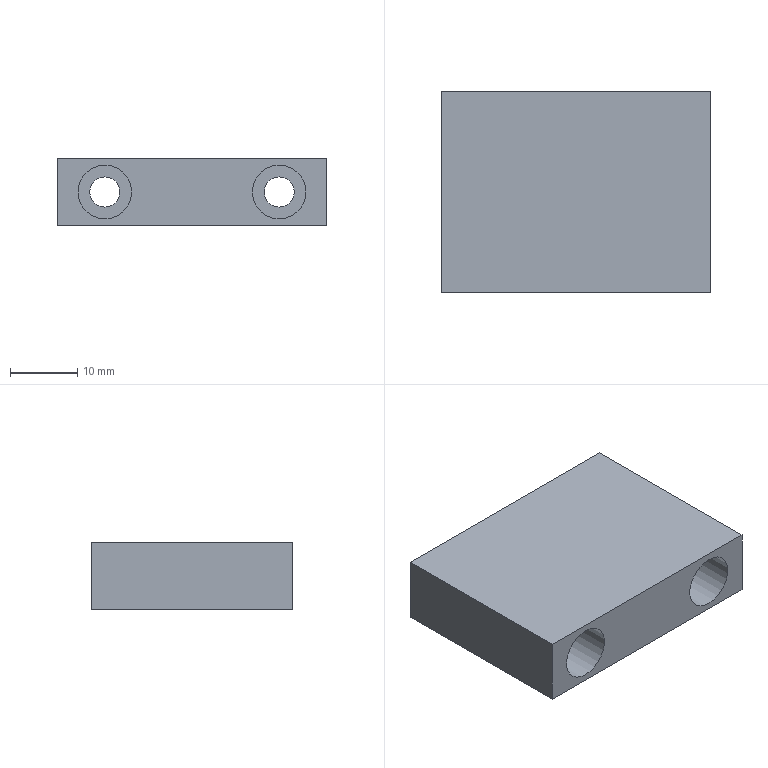Part | STEP file | 1 solid | 12 faces | box 40 x 30 x 10 mm | volume 9671 mm3 | plane 8 | cylinder 4 | commonest cylinder face diameters 4.5 x2 8 x2
STEP:
#1=CARTESIAN_POINT('',(0.,0.,0.));
#2=DIRECTION('',(0.,0.,1.));
#3=DIRECTION('',(1.,0.,0.));
#4=AXIS2_PLACEMENT_3D('',#1,#2,#3);
#5=CARTESIAN_POINT('',(-20.,15.,5.));
#6=VERTEX_POINT('',#5);
#7=CARTESIAN_POINT('',(20.,15.,5.));
#8=VERTEX_POINT('',#7);
#9=CARTESIAN_POINT('',(0.,15.,5.));
#10=DIRECTION('',(1.,0.,0.));
#11=VECTOR('',#10,1.);
#12=LINE('',#9,#11);
#13=CARTESIAN_POINT('',(0.,0.,5.));
#14=DIRECTION('',(0.,0.,-1.));
#15=DIRECTION('',(-1.,0.,0.));
#16=AXIS2_PLACEMENT_3D('',#13,#14,#15);
#17=PLANE('',#16);
#18=CARTESIAN_POINT('',(0.,15.));
#19=DIRECTION('',(-1.,0.));
#20=VECTOR('',#19,1.);
#21=LINE('',#18,#20);
#22=(GEOMETRIC_REPRESENTATION_CONTEXT(2)PARAMETRIC_REPRESENTATION_CONTEXT()REPRESENTATION_CONTEXT('',''));
#23=DEFINITIONAL_REPRESENTATION('',(#21),#22);
#24=PCURVE('',#17,#23);
#25=CARTESIAN_POINT('',(-20.,15.,5.));
#26=DIRECTION('',(0.,-1.,0.));
#27=DIRECTION('',(0.,0.,-1.));
#28=AXIS2_PLACEMENT_3D('',#25,#26,#27);
#29=PLANE('',#28);
#30=CARTESIAN_POINT('',(0.,20.));
#31=DIRECTION('',(0.,1.));
#32=VECTOR('',#31,1.);
#33=LINE('',#30,#32);
#34=(GEOMETRIC_REPRESENTATION_CONTEXT(2)PARAMETRIC_REPRESENTATION_CONTEXT()REPRESENTATION_CONTEXT('',''));
#35=DEFINITIONAL_REPRESENTATION('',(#33),#34);
#36=PCURVE('',#29,#35);
#37=SURFACE_CURVE('',#12,(#24,#36),.PCURVE_S1.);
#38=EDGE_CURVE('',#6,#8,#37,.T.);
#39=ORIENTED_EDGE('',*,*,#38,.F.);
#40=CARTESIAN_POINT('',(-20.,-15.,5.));
#41=VERTEX_POINT('',#40);
#42=CARTESIAN_POINT('',(-20.,0.,5.));
#43=DIRECTION('',(0.,1.,0.));
#44=VECTOR('',#43,1.);
#45=LINE('',#42,#44);
#46=CARTESIAN_POINT('',(20.,0.));
#47=DIRECTION('',(0.,1.));
#48=VECTOR('',#47,1.);
#49=LINE('',#46,#48);
#50=(GEOMETRIC_REPRESENTATION_CONTEXT(2)PARAMETRIC_REPRESENTATION_CONTEXT()REPRESENTATION_CONTEXT('',''));
#51=DEFINITIONAL_REPRESENTATION('',(#49),#50);
#52=PCURVE('',#17,#51);
#53=CARTESIAN_POINT('',(-20.,-15.,5.));
#54=DIRECTION('',(1.,0.,0.));
#55=DIRECTION('',(0.,0.,-1.));
#56=AXIS2_PLACEMENT_3D('',#53,#54,#55);
#57=PLANE('',#56);
#58=CARTESIAN_POINT('',(0.,15.));
#59=DIRECTION('',(0.,1.));
#60=VECTOR('',#59,1.);
#61=LINE('',#58,#60);
#62=(GEOMETRIC_REPRESENTATION_CONTEXT(2)PARAMETRIC_REPRESENTATION_CONTEXT()REPRESENTATION_CONTEXT('',''));
#63=DEFINITIONAL_REPRESENTATION('',(#61),#62);
#64=PCURVE('',#57,#63);
#65=SURFACE_CURVE('',#45,(#52,#64),.PCURVE_S1.);
#66=EDGE_CURVE('',#41,#6,#65,.T.);
#67=ORIENTED_EDGE('',*,*,#66,.F.);
#68=CARTESIAN_POINT('',(20.,-15.,5.));
#69=VERTEX_POINT('',#68);
#70=CARTESIAN_POINT('',(0.,-15.,5.));
#71=DIRECTION('',(-1.,0.,0.));
#72=VECTOR('',#71,1.);
#73=LINE('',#70,#72);
#74=CARTESIAN_POINT('',(0.,-15.));
#75=DIRECTION('',(1.,0.));
#76=VECTOR('',#75,1.);
#77=LINE('',#74,#76);
#78=(GEOMETRIC_REPRESENTATION_CONTEXT(2)PARAMETRIC_REPRESENTATION_CONTEXT()REPRESENTATION_CONTEXT('',''));
#79=DEFINITIONAL_REPRESENTATION('',(#77),#78);
#80=PCURVE('',#17,#79);
#81=CARTESIAN_POINT('',(-20.,-15.,5.));
#82=DIRECTION('',(0.,1.,0.));
#83=DIRECTION('',(0.,0.,1.));
#84=AXIS2_PLACEMENT_3D('',#81,#82,#83);
#85=PLANE('',#84);
#86=CARTESIAN_POINT('',(0.,20.));
#87=DIRECTION('',(0.,-1.));
#88=VECTOR('',#87,1.);
#89=LINE('',#86,#88);
#90=(GEOMETRIC_REPRESENTATION_CONTEXT(2)PARAMETRIC_REPRESENTATION_CONTEXT()REPRESENTATION_CONTEXT('',''));
#91=DEFINITIONAL_REPRESENTATION('',(#89),#90);
#92=PCURVE('',#85,#91);
#93=SURFACE_CURVE('',#73,(#80,#92),.PCURVE_S1.);
#94=EDGE_CURVE('',#69,#41,#93,.T.);
#95=ORIENTED_EDGE('',*,*,#94,.F.);
#96=CARTESIAN_POINT('',(20.,0.,5.));
#97=DIRECTION('',(0.,-1.,0.));
#98=VECTOR('',#97,1.);
#99=LINE('',#96,#98);
#100=CARTESIAN_POINT('',(-20.,0.));
#101=DIRECTION('',(0.,-1.));
#102=VECTOR('',#101,1.);
#103=LINE('',#100,#102);
#104=(GEOMETRIC_REPRESENTATION_CONTEXT(2)PARAMETRIC_REPRESENTATION_CONTEXT()REPRESENTATION_CONTEXT('',''));
#105=DEFINITIONAL_REPRESENTATION('',(#103),#104);
#106=PCURVE('',#17,#105);
#107=CARTESIAN_POINT('',(20.,-15.,5.));
#108=DIRECTION('',(-1.,0.,0.));
#109=DIRECTION('',(0.,0.,1.));
#110=AXIS2_PLACEMENT_3D('',#107,#108,#109);
#111=PLANE('',#110);
#112=CARTESIAN_POINT('',(0.,15.));
#113=DIRECTION('',(0.,-1.));
#114=VECTOR('',#113,1.);
#115=LINE('',#112,#114);
#116=(GEOMETRIC_REPRESENTATION_CONTEXT(2)PARAMETRIC_REPRESENTATION_CONTEXT()REPRESENTATION_CONTEXT('',''));
#117=DEFINITIONAL_REPRESENTATION('',(#115),#116);
#118=PCURVE('',#111,#117);
#119=SURFACE_CURVE('',#99,(#106,#118),.PCURVE_S1.);
#120=EDGE_CURVE('',#8,#69,#119,.T.);
#121=ORIENTED_EDGE('',*,*,#120,.F.);
#122=EDGE_LOOP('',(#39,#67,#95,#121));
#123=FACE_BOUND('',#122,.T.);
#124=ADVANCED_FACE('',(#123),#17,.F.);
#125=CARTESIAN_POINT('',(20.,15.,-5.));
#126=VERTEX_POINT('',#125);
#127=CARTESIAN_POINT('',(20.,15.,5.));
#128=DIRECTION('',(0.,0.,-1.));
#129=VECTOR('',#128,1.);
#130=LINE('',#127,#129);
#131=CARTESIAN_POINT('',(0.,30.));
#132=DIRECTION('',(-1.,0.));
#133=VECTOR('',#132,1.);
#134=LINE('',#131,#133);
#135=(GEOMETRIC_REPRESENTATION_CONTEXT(2)PARAMETRIC_REPRESENTATION_CONTEXT()REPRESENTATION_CONTEXT('',''));
#136=DEFINITIONAL_REPRESENTATION('',(#134),#135);
#137=PCURVE('',#111,#136);
#138=CARTESIAN_POINT('',(0.,40.));
#139=DIRECTION('',(1.,0.));
#140=VECTOR('',#139,1.);
#141=LINE('',#138,#140);
#142=(GEOMETRIC_REPRESENTATION_CONTEXT(2)PARAMETRIC_REPRESENTATION_CONTEXT()REPRESENTATION_CONTEXT('',''));
#143=DEFINITIONAL_REPRESENTATION('',(#141),#142);
#144=PCURVE('',#29,#143);
#145=SURFACE_CURVE('',#130,(#137,#144),.PCURVE_S1.);
#146=EDGE_CURVE('',#8,#126,#145,.T.);
#147=ORIENTED_EDGE('',*,*,#146,.F.);
#148=ORIENTED_EDGE('',*,*,#120,.T.);
#149=CARTESIAN_POINT('',(20.,-15.,-5.));
#150=VERTEX_POINT('',#149);
#151=CARTESIAN_POINT('',(20.,-15.,5.));
#152=DIRECTION('',(0.,0.,1.));
#153=VECTOR('',#152,1.);
#154=LINE('',#151,#153);
#155=CARTESIAN_POINT('',(0.,0.));
#156=DIRECTION('',(1.,0.));
#157=VECTOR('',#156,1.);
#158=LINE('',#155,#157);
#159=(GEOMETRIC_REPRESENTATION_CONTEXT(2)PARAMETRIC_REPRESENTATION_CONTEXT()REPRESENTATION_CONTEXT('',''));
#160=DEFINITIONAL_REPRESENTATION('',(#158),#159);
#161=PCURVE('',#111,#160);
#162=CARTESIAN_POINT('',(0.,40.));
#163=DIRECTION('',(1.,0.));
#164=VECTOR('',#163,1.);
#165=LINE('',#162,#164);
#166=(GEOMETRIC_REPRESENTATION_CONTEXT(2)PARAMETRIC_REPRESENTATION_CONTEXT()REPRESENTATION_CONTEXT('',''));
#167=DEFINITIONAL_REPRESENTATION('',(#165),#166);
#168=PCURVE('',#85,#167);
#169=SURFACE_CURVE('',#154,(#161,#168),.PCURVE_S1.);
#170=EDGE_CURVE('',#150,#69,#169,.T.);
#171=ORIENTED_EDGE('',*,*,#170,.F.);
#172=CARTESIAN_POINT('',(20.,-15.,-5.));
#173=DIRECTION('',(0.,-1.,0.));
#174=VECTOR('',#173,1.);
#175=LINE('',#172,#174);
#176=CARTESIAN_POINT('',(-10.,0.));
#177=DIRECTION('',(0.,-1.));
#178=VECTOR('',#177,1.);
#179=LINE('',#176,#178);
#180=(GEOMETRIC_REPRESENTATION_CONTEXT(2)PARAMETRIC_REPRESENTATION_CONTEXT()REPRESENTATION_CONTEXT('',''));
#181=DEFINITIONAL_REPRESENTATION('',(#179),#180);
#182=PCURVE('',#111,#181);
#183=CARTESIAN_POINT('',(0.,0.,-5.));
#184=DIRECTION('',(0.,0.,-1.));
#185=DIRECTION('',(-1.,0.,0.));
#186=AXIS2_PLACEMENT_3D('',#183,#184,#185);
#187=PLANE('',#186);
#188=CARTESIAN_POINT('',(-20.,-15.));
#189=DIRECTION('',(0.,-1.));
#190=VECTOR('',#189,1.);
#191=LINE('',#188,#190);
#192=(GEOMETRIC_REPRESENTATION_CONTEXT(2)PARAMETRIC_REPRESENTATION_CONTEXT()REPRESENTATION_CONTEXT('',''));
#193=DEFINITIONAL_REPRESENTATION('',(#191),#192);
#194=PCURVE('',#187,#193);
#195=SURFACE_CURVE('',#175,(#182,#194),.PCURVE_S1.);
#196=EDGE_CURVE('',#126,#150,#195,.T.);
#197=ORIENTED_EDGE('',*,*,#196,.F.);
#198=EDGE_LOOP('',(#147,#148,#171,#197));
#199=FACE_BOUND('',#198,.T.);
#200=ADVANCED_FACE('',(#199),#111,.F.);
#201=CARTESIAN_POINT('',(13.,15.,-2.25));
#202=VERTEX_POINT('',#201);
#203=CARTESIAN_POINT('',(13.,15.,0.));
#204=DIRECTION('',(0.,1.,0.));
#205=DIRECTION('',(0.,0.,-1.));
#206=AXIS2_PLACEMENT_3D('',#203,#204,#205);
#207=CIRCLE('',#206,2.25);
#208=CARTESIAN_POINT('',(7.25,33.));
#209=CARTESIAN_POINT('',(7.25,29.103));
#210=CARTESIAN_POINT('',(3.875,31.051));
#211=CARTESIAN_POINT('',(0.5,33.));
#212=CARTESIAN_POINT('',(3.875,34.949));
#213=CARTESIAN_POINT('',(7.25,36.897));
#214=CARTESIAN_POINT('',(7.25,33.));
#215=(BOUNDED_CURVE()B_SPLINE_CURVE(2,(#208,#209,#210,#211,#212,#213,#214),.UNSPECIFIED.,.T.,.F.)B_SPLINE_CURVE_WITH_KNOTS((1,2,2,2,2,1),(-2.094,0.,2.094,4.189,6.283,8.378),.UNSPECIFIED.)CURVE()GEOMETRIC_REPRESENTATION_ITEM()RATIONAL_B_SPLINE_CURVE((1.,0.5,1.,0.5,1.,0.5,1.))REPRESENTATION_ITEM(''));
#216=(GEOMETRIC_REPRESENTATION_CONTEXT(2)PARAMETRIC_REPRESENTATION_CONTEXT()REPRESENTATION_CONTEXT('',''));
#217=DEFINITIONAL_REPRESENTATION('',(#215),#216);
#218=PCURVE('',#29,#217);
#219=CARTESIAN_POINT('',(13.,-15.,0.));
#220=DIRECTION('',(0.,-1.,0.));
#221=DIRECTION('',(0.,0.,-1.));
#222=AXIS2_PLACEMENT_3D('',#219,#220,#221);
#223=CYLINDRICAL_SURFACE('',#222,2.25);
#224=CARTESIAN_POINT('',(6.283,-30.));
#225=DIRECTION('',(-1.,0.));
#226=VECTOR('',#225,1.);
#227=LINE('',#224,#226);
#228=(GEOMETRIC_REPRESENTATION_CONTEXT(2)PARAMETRIC_REPRESENTATION_CONTEXT()REPRESENTATION_CONTEXT('',''));
#229=DEFINITIONAL_REPRESENTATION('',(#227),#228);
#230=PCURVE('',#223,#229);
#231=SURFACE_CURVE('',#207,(#218,#230),.PCURVE_S1.);
#232=EDGE_CURVE('',#202,#202,#231,.T.);
#233=ORIENTED_EDGE('',*,*,#232,.F.);
#234=EDGE_LOOP('',(#233));
#235=FACE_BOUND('',#234,.T.);
#236=CARTESIAN_POINT('',(-13.,15.,-2.25));
#237=VERTEX_POINT('',#236);
#238=CARTESIAN_POINT('',(-13.,15.,0.));
#239=DIRECTION('',(0.,1.,0.));
#240=DIRECTION('',(0.,0.,-1.));
#241=AXIS2_PLACEMENT_3D('',#238,#239,#240);
#242=CIRCLE('',#241,2.25);
#243=CARTESIAN_POINT('',(7.25,7.));
#244=CARTESIAN_POINT('',(7.25,3.103));
#245=CARTESIAN_POINT('',(3.875,5.051));
#246=CARTESIAN_POINT('',(0.5,7.));
#247=CARTESIAN_POINT('',(3.875,8.949));
#248=CARTESIAN_POINT('',(7.25,10.897));
#249=CARTESIAN_POINT('',(7.25,7.));
#250=(BOUNDED_CURVE()B_SPLINE_CURVE(2,(#243,#244,#245,#246,#247,#248,#249),.UNSPECIFIED.,.T.,.F.)B_SPLINE_CURVE_WITH_KNOTS((1,2,2,2,2,1),(-2.094,0.,2.094,4.189,6.283,8.378),.UNSPECIFIED.)CURVE()GEOMETRIC_REPRESENTATION_ITEM()RATIONAL_B_SPLINE_CURVE((1.,0.5,1.,0.5,1.,0.5,1.))REPRESENTATION_ITEM(''));
#251=(GEOMETRIC_REPRESENTATION_CONTEXT(2)PARAMETRIC_REPRESENTATION_CONTEXT()REPRESENTATION_CONTEXT('',''));
#252=DEFINITIONAL_REPRESENTATION('',(#250),#251);
#253=PCURVE('',#29,#252);
#254=CARTESIAN_POINT('',(-13.,-15.,0.));
#255=DIRECTION('',(0.,-1.,0.));
#256=DIRECTION('',(0.,0.,-1.));
#257=AXIS2_PLACEMENT_3D('',#254,#255,#256);
#258=CYLINDRICAL_SURFACE('',#257,2.25);
#259=CARTESIAN_POINT('',(6.283,-30.));
#260=DIRECTION('',(-1.,0.));
#261=VECTOR('',#260,1.);
#262=LINE('',#259,#261);
#263=(GEOMETRIC_REPRESENTATION_CONTEXT(2)PARAMETRIC_REPRESENTATION_CONTEXT()REPRESENTATION_CONTEXT('',''));
#264=DEFINITIONAL_REPRESENTATION('',(#262),#263);
#265=PCURVE('',#258,#264);
#266=SURFACE_CURVE('',#242,(#253,#265),.PCURVE_S1.);
#267=EDGE_CURVE('',#237,#237,#266,.T.);
#268=ORIENTED_EDGE('',*,*,#267,.F.);
#269=EDGE_LOOP('',(#268));
#270=FACE_BOUND('',#269,.T.);
#271=CARTESIAN_POINT('',(-20.,15.,-5.));
#272=VERTEX_POINT('',#271);
#273=CARTESIAN_POINT('',(-20.,15.,5.));
#274=DIRECTION('',(0.,0.,-1.));
#275=VECTOR('',#274,1.);
#276=LINE('',#273,#275);
#277=CARTESIAN_POINT('',(0.,0.));
#278=DIRECTION('',(1.,0.));
#279=VECTOR('',#278,1.);
#280=LINE('',#277,#279);
#281=(GEOMETRIC_REPRESENTATION_CONTEXT(2)PARAMETRIC_REPRESENTATION_CONTEXT()REPRESENTATION_CONTEXT('',''));
#282=DEFINITIONAL_REPRESENTATION('',(#280),#281);
#283=PCURVE('',#29,#282);
#284=CARTESIAN_POINT('',(0.,30.));
#285=DIRECTION('',(1.,0.));
#286=VECTOR('',#285,1.);
#287=LINE('',#284,#286);
#288=(GEOMETRIC_REPRESENTATION_CONTEXT(2)PARAMETRIC_REPRESENTATION_CONTEXT()REPRESENTATION_CONTEXT('',''));
#289=DEFINITIONAL_REPRESENTATION('',(#287),#288);
#290=PCURVE('',#57,#289);
#291=SURFACE_CURVE('',#276,(#283,#290),.PCURVE_S1.);
#292=EDGE_CURVE('',#6,#272,#291,.T.);
#293=ORIENTED_EDGE('',*,*,#292,.F.);
#294=ORIENTED_EDGE('',*,*,#38,.T.);
#295=ORIENTED_EDGE('',*,*,#146,.T.);
#296=CARTESIAN_POINT('',(-20.,15.,-5.));
#297=DIRECTION('',(1.,0.,0.));
#298=VECTOR('',#297,1.);
#299=LINE('',#296,#298);
#300=CARTESIAN_POINT('',(10.,0.));
#301=DIRECTION('',(0.,1.));
#302=VECTOR('',#301,1.);
#303=LINE('',#300,#302);
#304=(GEOMETRIC_REPRESENTATION_CONTEXT(2)PARAMETRIC_REPRESENTATION_CONTEXT()REPRESENTATION_CONTEXT('',''));
#305=DEFINITIONAL_REPRESENTATION('',(#303),#304);
#306=PCURVE('',#29,#305);
#307=CARTESIAN_POINT('',(20.,15.));
#308=DIRECTION('',(-1.,0.));
#309=VECTOR('',#308,1.);
#310=LINE('',#307,#309);
#311=(GEOMETRIC_REPRESENTATION_CONTEXT(2)PARAMETRIC_REPRESENTATION_CONTEXT()REPRESENTATION_CONTEXT('',''));
#312=DEFINITIONAL_REPRESENTATION('',(#310),#311);
#313=PCURVE('',#187,#312);
#314=SURFACE_CURVE('',#299,(#306,#313),.PCURVE_S1.);
#315=EDGE_CURVE('',#272,#126,#314,.T.);
#316=ORIENTED_EDGE('',*,*,#315,.F.);
#317=EDGE_LOOP('',(#293,#294,#295,#316));
#318=FACE_BOUND('',#317,.T.);
#319=ADVANCED_FACE('',(#235,#270,#318),#29,.F.);
#320=CARTESIAN_POINT('',(-20.,-15.,-5.));
#321=VERTEX_POINT('',#320);
#322=CARTESIAN_POINT('',(-20.,-15.,5.));
#323=DIRECTION('',(0.,0.,-1.));
#324=VECTOR('',#323,1.);
#325=LINE('',#322,#324);
#326=CARTESIAN_POINT('',(0.,0.));
#327=DIRECTION('',(1.,0.));
#328=VECTOR('',#327,1.);
#329=LINE('',#326,#328);
#330=(GEOMETRIC_REPRESENTATION_CONTEXT(2)PARAMETRIC_REPRESENTATION_CONTEXT()REPRESENTATION_CONTEXT('',''));
#331=DEFINITIONAL_REPRESENTATION('',(#329),#330);
#332=PCURVE('',#57,#331);
#333=CARTESIAN_POINT('',(0.,0.));
#334=DIRECTION('',(-1.,0.));
#335=VECTOR('',#334,1.);
#336=LINE('',#333,#335);
#337=(GEOMETRIC_REPRESENTATION_CONTEXT(2)PARAMETRIC_REPRESENTATION_CONTEXT()REPRESENTATION_CONTEXT('',''));
#338=DEFINITIONAL_REPRESENTATION('',(#336),#337);
#339=PCURVE('',#85,#338);
#340=SURFACE_CURVE('',#325,(#332,#339),.PCURVE_S1.);
#341=EDGE_CURVE('',#41,#321,#340,.T.);
#342=ORIENTED_EDGE('',*,*,#341,.F.);
#343=ORIENTED_EDGE('',*,*,#66,.T.);
#344=ORIENTED_EDGE('',*,*,#292,.T.);
#345=CARTESIAN_POINT('',(-20.,-15.,-5.));
#346=DIRECTION('',(0.,1.,0.));
#347=VECTOR('',#346,1.);
#348=LINE('',#345,#347);
#349=CARTESIAN_POINT('',(10.,0.));
#350=DIRECTION('',(0.,1.));
#351=VECTOR('',#350,1.);
#352=LINE('',#349,#351);
#353=(GEOMETRIC_REPRESENTATION_CONTEXT(2)PARAMETRIC_REPRESENTATION_CONTEXT()REPRESENTATION_CONTEXT('',''));
#354=DEFINITIONAL_REPRESENTATION('',(#352),#353);
#355=PCURVE('',#57,#354);
#356=CARTESIAN_POINT('',(20.,-15.));
#357=DIRECTION('',(0.,1.));
#358=VECTOR('',#357,1.);
#359=LINE('',#356,#358);
#360=(GEOMETRIC_REPRESENTATION_CONTEXT(2)PARAMETRIC_REPRESENTATION_CONTEXT()REPRESENTATION_CONTEXT('',''));
#361=DEFINITIONAL_REPRESENTATION('',(#359),#360);
#362=PCURVE('',#187,#361);
#363=SURFACE_CURVE('',#348,(#355,#362),.PCURVE_S1.);
#364=EDGE_CURVE('',#321,#272,#363,.T.);
#365=ORIENTED_EDGE('',*,*,#364,.F.);
#366=EDGE_LOOP('',(#342,#343,#344,#365));
#367=FACE_BOUND('',#366,.T.);
#368=ADVANCED_FACE('',(#367),#57,.F.);
#369=CARTESIAN_POINT('',(13.,-15.,-4.));
#370=VERTEX_POINT('',#369);
#371=CARTESIAN_POINT('',(13.,-15.,0.));
#372=DIRECTION('',(0.,-1.,0.));
#373=DIRECTION('',(0.,0.,-1.));
#374=AXIS2_PLACEMENT_3D('',#371,#372,#373);
#375=CIRCLE('',#374,4.);
#376=CARTESIAN_POINT('',(-9.,33.));
#377=CARTESIAN_POINT('',(-9.,39.928));
#378=CARTESIAN_POINT('',(-3.,36.464));
#379=CARTESIAN_POINT('',(3.,33.));
#380=CARTESIAN_POINT('',(-3.,29.536));
#381=CARTESIAN_POINT('',(-9.,26.072));
#382=CARTESIAN_POINT('',(-9.,33.));
#383=(BOUNDED_CURVE()B_SPLINE_CURVE(2,(#376,#377,#378,#379,#380,#381,#382),.UNSPECIFIED.,.T.,.F.)B_SPLINE_CURVE_WITH_KNOTS((1,2,2,2,2,1),(-2.094,0.,2.094,4.189,6.283,8.378),.UNSPECIFIED.)CURVE()GEOMETRIC_REPRESENTATION_ITEM()RATIONAL_B_SPLINE_CURVE((1.,0.5,1.,0.5,1.,0.5,1.))REPRESENTATION_ITEM(''));
#384=(GEOMETRIC_REPRESENTATION_CONTEXT(2)PARAMETRIC_REPRESENTATION_CONTEXT()REPRESENTATION_CONTEXT('',''));
#385=DEFINITIONAL_REPRESENTATION('',(#383),#384);
#386=PCURVE('',#85,#385);
#387=CARTESIAN_POINT('',(13.,-15.,0.));
#388=DIRECTION('',(0.,-1.,0.));
#389=DIRECTION('',(0.,0.,-1.));
#390=AXIS2_PLACEMENT_3D('',#387,#388,#389);
#391=CYLINDRICAL_SURFACE('',#390,4.);
#392=CARTESIAN_POINT('',(0.,0.));
#393=DIRECTION('',(1.,0.));
#394=VECTOR('',#393,1.);
#395=LINE('',#392,#394);
#396=(GEOMETRIC_REPRESENTATION_CONTEXT(2)PARAMETRIC_REPRESENTATION_CONTEXT()REPRESENTATION_CONTEXT('',''));
#397=DEFINITIONAL_REPRESENTATION('',(#395),#396);
#398=PCURVE('',#391,#397);
#399=SURFACE_CURVE('',#375,(#386,#398),.PCURVE_S1.);
#400=EDGE_CURVE('',#370,#370,#399,.T.);
#401=ORIENTED_EDGE('',*,*,#400,.F.);
#402=EDGE_LOOP('',(#401));
#403=FACE_BOUND('',#402,.T.);
#404=CARTESIAN_POINT('',(-13.,-15.,-4.));
#405=VERTEX_POINT('',#404);
#406=CARTESIAN_POINT('',(-13.,-15.,0.));
#407=DIRECTION('',(0.,-1.,0.));
#408=DIRECTION('',(0.,0.,-1.));
#409=AXIS2_PLACEMENT_3D('',#406,#407,#408);
#410=CIRCLE('',#409,4.);
#411=CARTESIAN_POINT('',(-9.,7.));
#412=CARTESIAN_POINT('',(-9.,13.928));
#413=CARTESIAN_POINT('',(-3.,10.464));
#414=CARTESIAN_POINT('',(3.,7.));
#415=CARTESIAN_POINT('',(-3.,3.536));
#416=CARTESIAN_POINT('',(-9.,0.0718));
#417=CARTESIAN_POINT('',(-9.,7.));
#418=(BOUNDED_CURVE()B_SPLINE_CURVE(2,(#411,#412,#413,#414,#415,#416,#417),.UNSPECIFIED.,.T.,.F.)B_SPLINE_CURVE_WITH_KNOTS((1,2,2,2,2,1),(-2.094,0.,2.094,4.189,6.283,8.378),.UNSPECIFIED.)CURVE()GEOMETRIC_REPRESENTATION_ITEM()RATIONAL_B_SPLINE_CURVE((1.,0.5,1.,0.5,1.,0.5,1.))REPRESENTATION_ITEM(''));
#419=(GEOMETRIC_REPRESENTATION_CONTEXT(2)PARAMETRIC_REPRESENTATION_CONTEXT()REPRESENTATION_CONTEXT('',''));
#420=DEFINITIONAL_REPRESENTATION('',(#418),#419);
#421=PCURVE('',#85,#420);
#422=CARTESIAN_POINT('',(-13.,-15.,0.));
#423=DIRECTION('',(0.,-1.,0.));
#424=DIRECTION('',(0.,0.,-1.));
#425=AXIS2_PLACEMENT_3D('',#422,#423,#424);
#426=CYLINDRICAL_SURFACE('',#425,4.);
#427=CARTESIAN_POINT('',(0.,0.));
#428=DIRECTION('',(1.,0.));
#429=VECTOR('',#428,1.);
#430=LINE('',#427,#429);
#431=(GEOMETRIC_REPRESENTATION_CONTEXT(2)PARAMETRIC_REPRESENTATION_CONTEXT()REPRESENTATION_CONTEXT('',''));
#432=DEFINITIONAL_REPRESENTATION('',(#430),#431);
#433=PCURVE('',#426,#432);
#434=SURFACE_CURVE('',#410,(#421,#433),.PCURVE_S1.);
#435=EDGE_CURVE('',#405,#405,#434,.T.);
#436=ORIENTED_EDGE('',*,*,#435,.F.);
#437=EDGE_LOOP('',(#436));
#438=FACE_BOUND('',#437,.T.);
#439=ORIENTED_EDGE('',*,*,#170,.T.);
#440=ORIENTED_EDGE('',*,*,#94,.T.);
#441=ORIENTED_EDGE('',*,*,#341,.T.);
#442=CARTESIAN_POINT('',(-20.,-15.,-5.));
#443=DIRECTION('',(-1.,0.,0.));
#444=VECTOR('',#443,1.);
#445=LINE('',#442,#444);
#446=CARTESIAN_POINT('',(-10.,0.));
#447=DIRECTION('',(0.,-1.));
#448=VECTOR('',#447,1.);
#449=LINE('',#446,#448);
#450=(GEOMETRIC_REPRESENTATION_CONTEXT(2)PARAMETRIC_REPRESENTATION_CONTEXT()REPRESENTATION_CONTEXT('',''));
#451=DEFINITIONAL_REPRESENTATION('',(#449),#450);
#452=PCURVE('',#85,#451);
#453=CARTESIAN_POINT('',(20.,-15.));
#454=DIRECTION('',(1.,0.));
#455=VECTOR('',#454,1.);
#456=LINE('',#453,#455);
#457=(GEOMETRIC_REPRESENTATION_CONTEXT(2)PARAMETRIC_REPRESENTATION_CONTEXT()REPRESENTATION_CONTEXT('',''));
#458=DEFINITIONAL_REPRESENTATION('',(#456),#457);
#459=PCURVE('',#187,#458);
#460=SURFACE_CURVE('',#445,(#452,#459),.PCURVE_S1.);
#461=EDGE_CURVE('',#150,#321,#460,.T.);
#462=ORIENTED_EDGE('',*,*,#461,.F.);
#463=EDGE_LOOP('',(#439,#440,#441,#462));
#464=FACE_BOUND('',#463,.T.);
#465=ADVANCED_FACE('',(#403,#438,#464),#85,.F.);
#466=ORIENTED_EDGE('',*,*,#364,.T.);
#467=ORIENTED_EDGE('',*,*,#315,.T.);
#468=ORIENTED_EDGE('',*,*,#196,.T.);
#469=ORIENTED_EDGE('',*,*,#461,.T.);
#470=EDGE_LOOP('',(#466,#467,#468,#469));
#471=FACE_BOUND('',#470,.T.);
#472=ADVANCED_FACE('',(#471),#187,.T.);
#473=ORIENTED_EDGE('',*,*,#232,.F.);
#474=CARTESIAN_POINT('',(13.,5.,-2.25));
#475=VERTEX_POINT('',#474);
#476=CARTESIAN_POINT('',(13.,15.,-2.25));
#477=CARTESIAN_POINT('',(13.,5.,-2.25));
#478=B_SPLINE_CURVE_WITH_KNOTS('',1,(#476,#477),.UNSPECIFIED.,.F.,.F.,(2,2),(-30.,-20.),.PIECEWISE_BEZIER_KNOTS.);
#479=CARTESIAN_POINT('',(6.283,0.));
#480=DIRECTION('',(0.,1.));
#481=VECTOR('',#480,1.);
#482=LINE('',#479,#481);
#483=(GEOMETRIC_REPRESENTATION_CONTEXT(2)PARAMETRIC_REPRESENTATION_CONTEXT()REPRESENTATION_CONTEXT('',''));
#484=DEFINITIONAL_REPRESENTATION('',(#482),#483);
#485=PCURVE('',#223,#484);
#486=CARTESIAN_POINT('',(0.,0.));
#487=DIRECTION('',(0.,1.));
#488=VECTOR('',#487,1.);
#489=LINE('',#486,#488);
#490=(GEOMETRIC_REPRESENTATION_CONTEXT(2)PARAMETRIC_REPRESENTATION_CONTEXT()REPRESENTATION_CONTEXT('',''));
#491=DEFINITIONAL_REPRESENTATION('',(#489),#490);
#492=PCURVE('',#223,#491);
#493=SEAM_CURVE('',#478,(#485,#492),.PCURVE_S1.);
#494=EDGE_CURVE('',#202,#475,#493,.T.);
#495=ORIENTED_EDGE('',*,*,#494,.T.);
#496=CARTESIAN_POINT('',(13.,5.,0.));
#497=DIRECTION('',(0.,1.,0.));
#498=DIRECTION('',(0.,0.,-1.));
#499=AXIS2_PLACEMENT_3D('',#496,#497,#498);
#500=CIRCLE('',#499,2.25);
#501=CARTESIAN_POINT('',(6.283,-20.));
#502=DIRECTION('',(-1.,0.));
#503=VECTOR('',#502,1.);
#504=LINE('',#501,#503);
#505=(GEOMETRIC_REPRESENTATION_CONTEXT(2)PARAMETRIC_REPRESENTATION_CONTEXT()REPRESENTATION_CONTEXT('',''));
#506=DEFINITIONAL_REPRESENTATION('',(#504),#505);
#507=PCURVE('',#223,#506);
#508=CARTESIAN_POINT('',(15.25,5.,0.));
#509=DIRECTION('',(0.,1.,0.));
#510=DIRECTION('',(0.,0.,1.));
#511=AXIS2_PLACEMENT_3D('',#508,#509,#510);
#512=PLANE('',#511);
#513=CARTESIAN_POINT('',(0.,-2.25));
#514=DIRECTION('',(-1.,0.));
#515=AXIS2_PLACEMENT_2D('',#513,#514);
#516=CIRCLE('',#515,2.25);
#517=(GEOMETRIC_REPRESENTATION_CONTEXT(2)PARAMETRIC_REPRESENTATION_CONTEXT()REPRESENTATION_CONTEXT('',''));
#518=DEFINITIONAL_REPRESENTATION('',(#516),#517);
#519=PCURVE('',#512,#518);
#520=SURFACE_CURVE('',#500,(#507,#519),.PCURVE_S1.);
#521=EDGE_CURVE('',#475,#475,#520,.T.);
#522=ORIENTED_EDGE('',*,*,#521,.T.);
#523=ORIENTED_EDGE('',*,*,#494,.F.);
#524=EDGE_LOOP('',(#473,#495,#522,#523));
#525=FACE_BOUND('',#524,.F.);
#526=ADVANCED_FACE('',(#525),#223,.F.);
#527=ORIENTED_EDGE('',*,*,#267,.F.);
#528=CARTESIAN_POINT('',(-13.,5.,-2.25));
#529=VERTEX_POINT('',#528);
#530=CARTESIAN_POINT('',(-13.,15.,-2.25));
#531=CARTESIAN_POINT('',(-13.,5.,-2.25));
#532=B_SPLINE_CURVE_WITH_KNOTS('',1,(#530,#531),.UNSPECIFIED.,.F.,.F.,(2,2),(-30.,-20.),.PIECEWISE_BEZIER_KNOTS.);
#533=CARTESIAN_POINT('',(6.283,0.));
#534=DIRECTION('',(0.,1.));
#535=VECTOR('',#534,1.);
#536=LINE('',#533,#535);
#537=(GEOMETRIC_REPRESENTATION_CONTEXT(2)PARAMETRIC_REPRESENTATION_CONTEXT()REPRESENTATION_CONTEXT('',''));
#538=DEFINITIONAL_REPRESENTATION('',(#536),#537);
#539=PCURVE('',#258,#538);
#540=CARTESIAN_POINT('',(0.,0.));
#541=DIRECTION('',(0.,1.));
#542=VECTOR('',#541,1.);
#543=LINE('',#540,#542);
#544=(GEOMETRIC_REPRESENTATION_CONTEXT(2)PARAMETRIC_REPRESENTATION_CONTEXT()REPRESENTATION_CONTEXT('',''));
#545=DEFINITIONAL_REPRESENTATION('',(#543),#544);
#546=PCURVE('',#258,#545);
#547=SEAM_CURVE('',#532,(#539,#546),.PCURVE_S1.);
#548=EDGE_CURVE('',#237,#529,#547,.T.);
#549=ORIENTED_EDGE('',*,*,#548,.T.);
#550=CARTESIAN_POINT('',(-13.,5.,0.));
#551=DIRECTION('',(0.,1.,0.));
#552=DIRECTION('',(0.,0.,-1.));
#553=AXIS2_PLACEMENT_3D('',#550,#551,#552);
#554=CIRCLE('',#553,2.25);
#555=CARTESIAN_POINT('',(6.283,-20.));
#556=DIRECTION('',(-1.,0.));
#557=VECTOR('',#556,1.);
#558=LINE('',#555,#557);
#559=(GEOMETRIC_REPRESENTATION_CONTEXT(2)PARAMETRIC_REPRESENTATION_CONTEXT()REPRESENTATION_CONTEXT('',''));
#560=DEFINITIONAL_REPRESENTATION('',(#558),#559);
#561=PCURVE('',#258,#560);
#562=CARTESIAN_POINT('',(-10.75,5.,0.));
#563=DIRECTION('',(0.,1.,0.));
#564=DIRECTION('',(0.,0.,1.));
#565=AXIS2_PLACEMENT_3D('',#562,#563,#564);
#566=PLANE('',#565);
#567=CARTESIAN_POINT('',(0.,-2.25));
#568=DIRECTION('',(-1.,0.));
#569=AXIS2_PLACEMENT_2D('',#567,#568);
#570=CIRCLE('',#569,2.25);
#571=(GEOMETRIC_REPRESENTATION_CONTEXT(2)PARAMETRIC_REPRESENTATION_CONTEXT()REPRESENTATION_CONTEXT('',''));
#572=DEFINITIONAL_REPRESENTATION('',(#570),#571);
#573=PCURVE('',#566,#572);
#574=SURFACE_CURVE('',#554,(#561,#573),.PCURVE_S1.);
#575=EDGE_CURVE('',#529,#529,#574,.T.);
#576=ORIENTED_EDGE('',*,*,#575,.T.);
#577=ORIENTED_EDGE('',*,*,#548,.F.);
#578=EDGE_LOOP('',(#527,#549,#576,#577));
#579=FACE_BOUND('',#578,.F.);
#580=ADVANCED_FACE('',(#579),#258,.F.);
#581=CARTESIAN_POINT('',(13.,5.,-4.));
#582=VERTEX_POINT('',#581);
#583=CARTESIAN_POINT('',(13.,5.,0.));
#584=DIRECTION('',(0.,-1.,0.));
#585=DIRECTION('',(0.,0.,-1.));
#586=AXIS2_PLACEMENT_3D('',#583,#584,#585);
#587=CIRCLE('',#586,4.);
#588=CARTESIAN_POINT('',(0.,-20.));
#589=DIRECTION('',(1.,0.));
#590=VECTOR('',#589,1.);
#591=LINE('',#588,#590);
#592=(GEOMETRIC_REPRESENTATION_CONTEXT(2)PARAMETRIC_REPRESENTATION_CONTEXT()REPRESENTATION_CONTEXT('',''));
#593=DEFINITIONAL_REPRESENTATION('',(#591),#592);
#594=PCURVE('',#391,#593);
#595=CARTESIAN_POINT('',(-4.,-2.25));
#596=CARTESIAN_POINT('',(-4.,4.678));
#597=CARTESIAN_POINT('',(2.,1.214));
#598=CARTESIAN_POINT('',(8.,-2.25));
#599=CARTESIAN_POINT('',(2.,-5.714));
#600=CARTESIAN_POINT('',(-4.,-9.178));
#601=CARTESIAN_POINT('',(-4.,-2.25));
#602=(BOUNDED_CURVE()B_SPLINE_CURVE(2,(#595,#596,#597,#598,#599,#600,#601),.UNSPECIFIED.,.T.,.F.)B_SPLINE_CURVE_WITH_KNOTS((1,2,2,2,2,1),(-2.094,0.,2.094,4.189,6.283,8.378),.UNSPECIFIED.)CURVE()GEOMETRIC_REPRESENTATION_ITEM()RATIONAL_B_SPLINE_CURVE((1.,0.5,1.,0.5,1.,0.5,1.))REPRESENTATION_ITEM(''));
#603=(GEOMETRIC_REPRESENTATION_CONTEXT(2)PARAMETRIC_REPRESENTATION_CONTEXT()REPRESENTATION_CONTEXT('',''));
#604=DEFINITIONAL_REPRESENTATION('',(#602),#603);
#605=PCURVE('',#512,#604);
#606=SURFACE_CURVE('',#587,(#594,#605),.PCURVE_S1.);
#607=EDGE_CURVE('',#582,#582,#606,.T.);
#608=ORIENTED_EDGE('',*,*,#607,.T.);
#609=CARTESIAN_POINT('',(13.,5.,-4.));
#610=CARTESIAN_POINT('',(13.,-15.,-4.));
#611=B_SPLINE_CURVE_WITH_KNOTS('',1,(#609,#610),.UNSPECIFIED.,.F.,.F.,(2,2),(-20.,0.),.PIECEWISE_BEZIER_KNOTS.);
#612=CARTESIAN_POINT('',(6.283,0.));
#613=DIRECTION('',(0.,1.));
#614=VECTOR('',#613,1.);
#615=LINE('',#612,#614);
#616=(GEOMETRIC_REPRESENTATION_CONTEXT(2)PARAMETRIC_REPRESENTATION_CONTEXT()REPRESENTATION_CONTEXT('',''));
#617=DEFINITIONAL_REPRESENTATION('',(#615),#616);
#618=PCURVE('',#391,#617);
#619=CARTESIAN_POINT('',(0.,0.));
#620=DIRECTION('',(0.,1.));
#621=VECTOR('',#620,1.);
#622=LINE('',#619,#621);
#623=(GEOMETRIC_REPRESENTATION_CONTEXT(2)PARAMETRIC_REPRESENTATION_CONTEXT()REPRESENTATION_CONTEXT('',''));
#624=DEFINITIONAL_REPRESENTATION('',(#622),#623);
#625=PCURVE('',#391,#624);
#626=SEAM_CURVE('',#611,(#618,#625),.PCURVE_S1.);
#627=EDGE_CURVE('',#582,#370,#626,.T.);
#628=ORIENTED_EDGE('',*,*,#627,.T.);
#629=ORIENTED_EDGE('',*,*,#400,.F.);
#630=ORIENTED_EDGE('',*,*,#627,.F.);
#631=EDGE_LOOP('',(#608,#628,#629,#630));
#632=FACE_BOUND('',#631,.F.);
#633=ADVANCED_FACE('',(#632),#391,.F.);
#634=CARTESIAN_POINT('',(-13.,5.,-4.));
#635=VERTEX_POINT('',#634);
#636=CARTESIAN_POINT('',(-13.,5.,0.));
#637=DIRECTION('',(0.,-1.,0.));
#638=DIRECTION('',(0.,0.,-1.));
#639=AXIS2_PLACEMENT_3D('',#636,#637,#638);
#640=CIRCLE('',#639,4.);
#641=CARTESIAN_POINT('',(0.,-20.));
#642=DIRECTION('',(1.,0.));
#643=VECTOR('',#642,1.);
#644=LINE('',#641,#643);
#645=(GEOMETRIC_REPRESENTATION_CONTEXT(2)PARAMETRIC_REPRESENTATION_CONTEXT()REPRESENTATION_CONTEXT('',''));
#646=DEFINITIONAL_REPRESENTATION('',(#644),#645);
#647=PCURVE('',#426,#646);
#648=CARTESIAN_POINT('',(-4.,-2.25));
#649=CARTESIAN_POINT('',(-4.,4.678));
#650=CARTESIAN_POINT('',(2.,1.214));
#651=CARTESIAN_POINT('',(8.,-2.25));
#652=CARTESIAN_POINT('',(2.,-5.714));
#653=CARTESIAN_POINT('',(-4.,-9.178));
#654=CARTESIAN_POINT('',(-4.,-2.25));
#655=(BOUNDED_CURVE()B_SPLINE_CURVE(2,(#648,#649,#650,#651,#652,#653,#654),.UNSPECIFIED.,.T.,.F.)B_SPLINE_CURVE_WITH_KNOTS((1,2,2,2,2,1),(-2.094,0.,2.094,4.189,6.283,8.378),.UNSPECIFIED.)CURVE()GEOMETRIC_REPRESENTATION_ITEM()RATIONAL_B_SPLINE_CURVE((1.,0.5,1.,0.5,1.,0.5,1.))REPRESENTATION_ITEM(''));
#656=(GEOMETRIC_REPRESENTATION_CONTEXT(2)PARAMETRIC_REPRESENTATION_CONTEXT()REPRESENTATION_CONTEXT('',''));
#657=DEFINITIONAL_REPRESENTATION('',(#655),#656);
#658=PCURVE('',#566,#657);
#659=SURFACE_CURVE('',#640,(#647,#658),.PCURVE_S1.);
#660=EDGE_CURVE('',#635,#635,#659,.T.);
#661=ORIENTED_EDGE('',*,*,#660,.T.);
#662=CARTESIAN_POINT('',(-13.,5.,-4.));
#663=CARTESIAN_POINT('',(-13.,-15.,-4.));
#664=B_SPLINE_CURVE_WITH_KNOTS('',1,(#662,#663),.UNSPECIFIED.,.F.,.F.,(2,2),(-20.,0.),.PIECEWISE_BEZIER_KNOTS.);
#665=CARTESIAN_POINT('',(6.283,0.));
#666=DIRECTION('',(0.,1.));
#667=VECTOR('',#666,1.);
#668=LINE('',#665,#667);
#669=(GEOMETRIC_REPRESENTATION_CONTEXT(2)PARAMETRIC_REPRESENTATION_CONTEXT()REPRESENTATION_CONTEXT('',''));
#670=DEFINITIONAL_REPRESENTATION('',(#668),#669);
#671=PCURVE('',#426,#670);
#672=CARTESIAN_POINT('',(0.,0.));
#673=DIRECTION('',(0.,1.));
#674=VECTOR('',#673,1.);
#675=LINE('',#672,#674);
#676=(GEOMETRIC_REPRESENTATION_CONTEXT(2)PARAMETRIC_REPRESENTATION_CONTEXT()REPRESENTATION_CONTEXT('',''));
#677=DEFINITIONAL_REPRESENTATION('',(#675),#676);
#678=PCURVE('',#426,#677);
#679=SEAM_CURVE('',#664,(#671,#678),.PCURVE_S1.);
#680=EDGE_CURVE('',#635,#405,#679,.T.);
#681=ORIENTED_EDGE('',*,*,#680,.T.);
#682=ORIENTED_EDGE('',*,*,#435,.F.);
#683=ORIENTED_EDGE('',*,*,#680,.F.);
#684=EDGE_LOOP('',(#661,#681,#682,#683));
#685=FACE_BOUND('',#684,.F.);
#686=ADVANCED_FACE('',(#685),#426,.F.);
#687=ORIENTED_EDGE('',*,*,#521,.T.);
#688=EDGE_LOOP('',(#687));
#689=FACE_BOUND('',#688,.T.);
#690=ORIENTED_EDGE('',*,*,#607,.T.);
#691=EDGE_LOOP('',(#690));
#692=FACE_BOUND('',#691,.T.);
#693=ADVANCED_FACE('',(#689,#692),#512,.F.);
#694=ORIENTED_EDGE('',*,*,#575,.T.);
#695=EDGE_LOOP('',(#694));
#696=FACE_BOUND('',#695,.T.);
#697=ORIENTED_EDGE('',*,*,#660,.T.);
#698=EDGE_LOOP('',(#697));
#699=FACE_BOUND('',#698,.T.);
#700=ADVANCED_FACE('',(#696,#699),#566,.F.);
#701=CLOSED_SHELL('',(#124,#200,#319,#368,#465,#472,#526,#580,#633,#686,#693,#700));
#702=MANIFOLD_SOLID_BREP('',#701);
#703=(LENGTH_UNIT()NAMED_UNIT(*)SI_UNIT(.MILLI.,.METRE.));
#704=UNCERTAINTY_MEASURE_WITH_UNIT(LENGTH_MEASURE(0.000005),#703,'','');
#705=(NAMED_UNIT(*)PLANE_ANGLE_UNIT()SI_UNIT($,.RADIAN.));
#706=(NAMED_UNIT(*)SI_UNIT($,.STERADIAN.)SOLID_ANGLE_UNIT());
#707=(GEOMETRIC_REPRESENTATION_CONTEXT(3)GLOBAL_UNCERTAINTY_ASSIGNED_CONTEXT((#704))GLOBAL_UNIT_ASSIGNED_CONTEXT((#703,#705,#706))REPRESENTATION_CONTEXT('',''));
#708=ADVANCED_BREP_SHAPE_REPRESENTATION('',(#4,#702),#707);